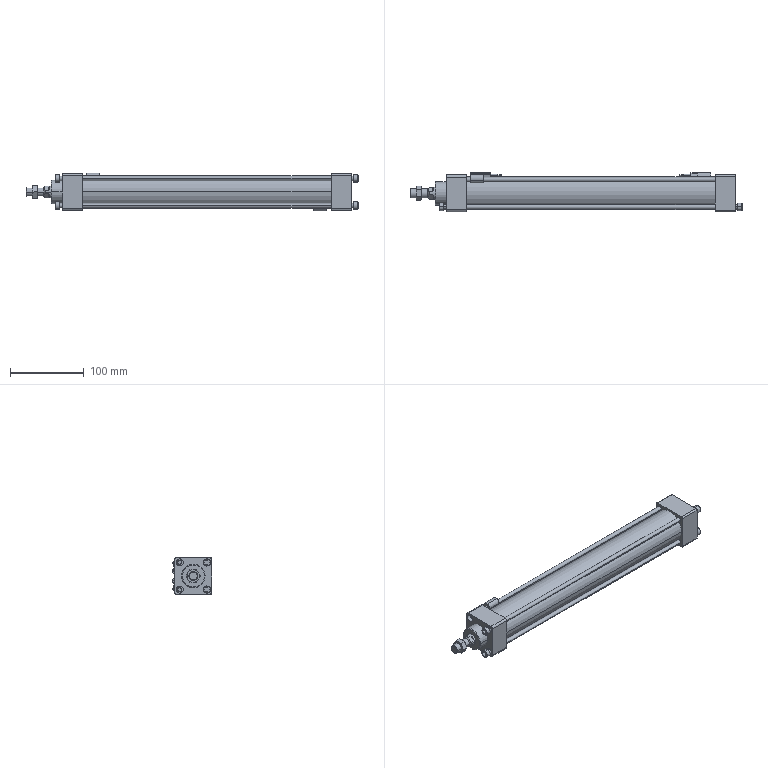Part | SolidWorks | 11 solids | 472 faces | box 451 x 53.518 x 51.2 mm | volume 402032 mm3 | plane 214 | cylinder 164 | cone 84 | torus 10 | commonest cylinder face diameters 6 x20 4.917 x16 9.5 x16 4 x14 10 x10 0.4 x8